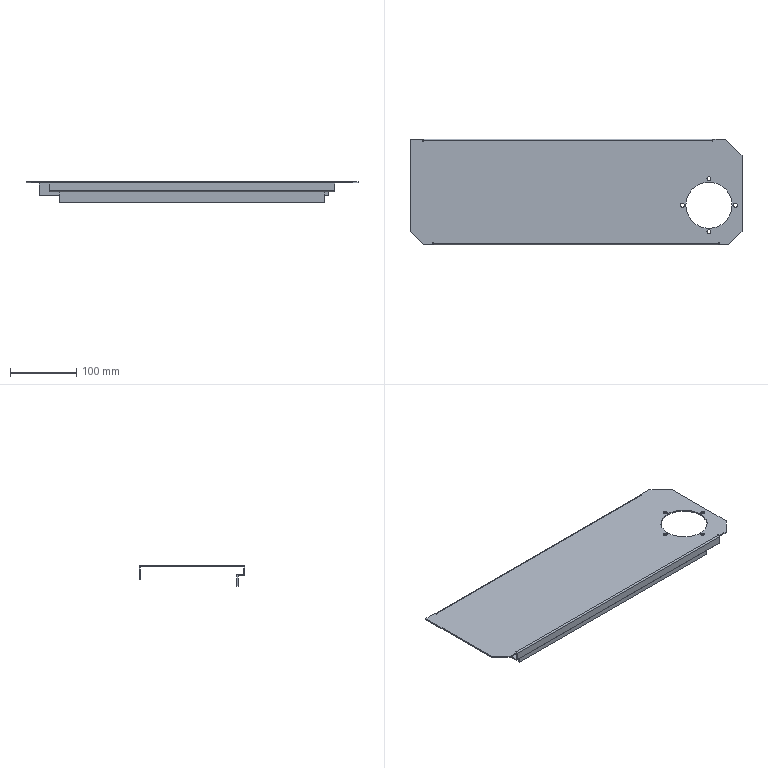Part | STEP file | Box Control Box | 1 solid | 59 faces | box 502 x 160 x 31.5 mm | volume 198922 mm3 | plane 41 | cylinder 18 | commonest cylinder face diameters 6 x8 0.2 x4 4.2 x4 70 x2